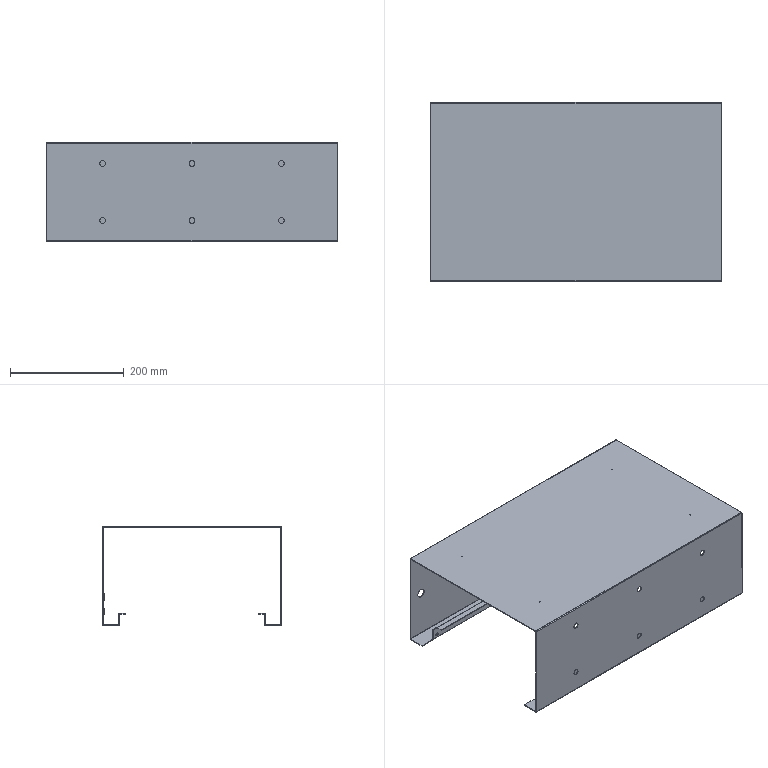Part | 1 solid | 166 faces | box 512 x 315 x 175 mm | volume 588332 mm3 | plane 94 | cylinder 72 | commonest cylinder face diameters 10 x12 16 x12 0.2 x8 2 x8 3.2 x8 5.2 x8